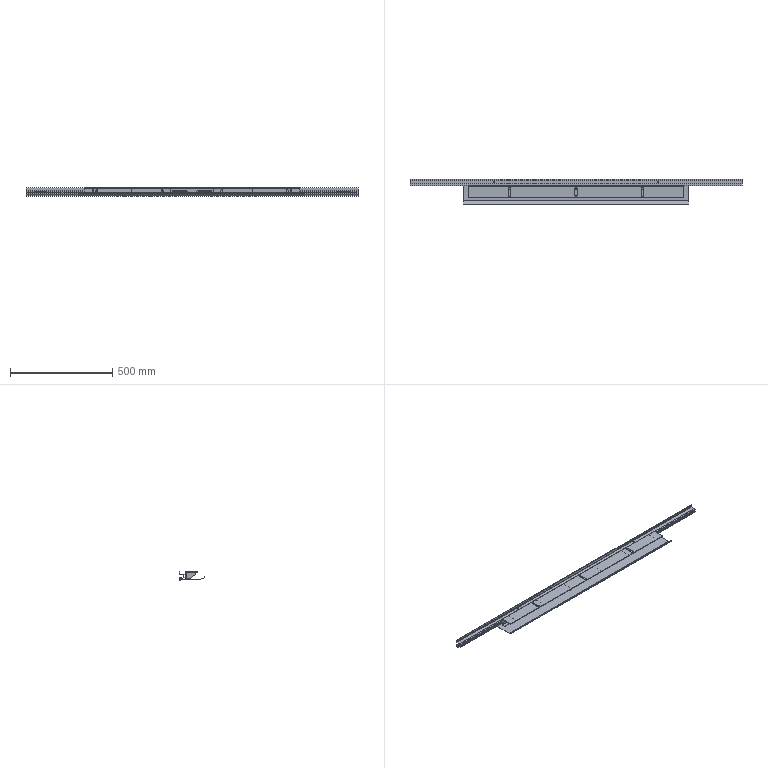Part | 9 solids | 263 faces | box 1620 x 122.321 x 40 mm | volume 788401 mm3 | plane 171 | cylinder 92 | commonest cylinder face diameters 9 x30 6 x25 10 x18 2 x9 12 x4 3 x2